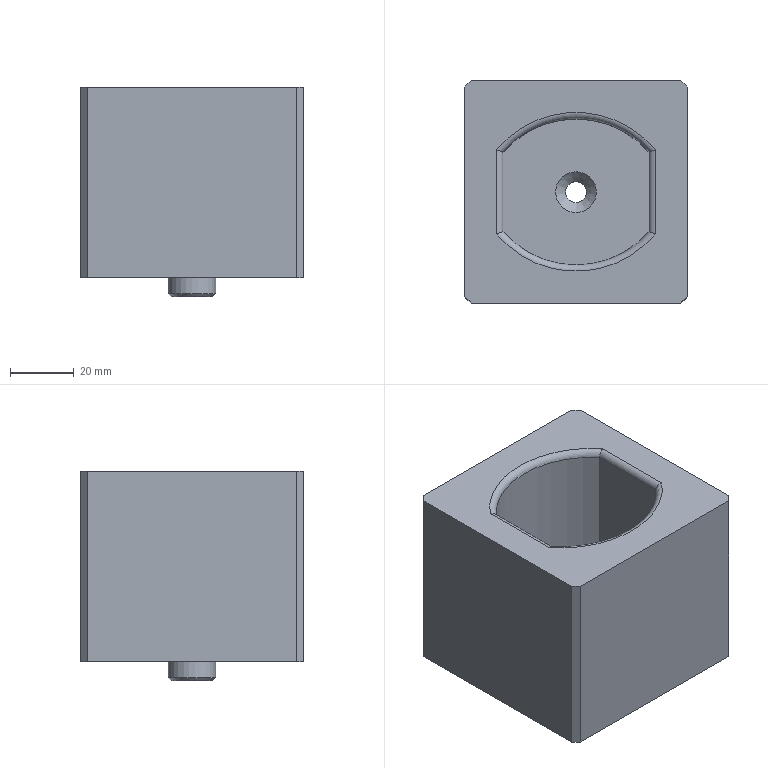NC program | NX | posted with a generic post | part box 70 x 70 x 66 mm
Lines 59 to 918 of 8582:
(ZLEVEL_PROFILE_COPY_1_COPY , TOOL : D16)
N116 T22 M6
N118 G54
N120 G17 G0 G90 X-8. Y-5.119 S7500 M3
N122 G43 Z30. H22
N124 Z1.4
N126 G94 G1 Y-5.61 Z1.374 F1000.
N128 X-8.004 Y-5.764 Z1.366
N130 X-7.18 Y-6.263 Z1.316
N132 X-4.893 Y-7.236 Z1.185
N134 X-2.48 Y-7.83 Z1.055
N136 X-0.002 Y-8.03 Z0.925
N138 X2.475 Y-7.83 Z0.795
N140 X4.889 Y-7.237 Z0.664
N142 X7.176 Y-6.265 Z0.534
N144 X8. Y-5.766 Z0.484
N146 Y5.764 Z-0.121
N148 X7.912 Y5.819 Z-0.126
N150 X7.084 Y6.312 Z-0.176
N152 X4.825 Y7.258 Z-0.305
N154 X2.444 Y7.835 Z-0.433
N156 X0.002 Y8.03 Z-0.562
N158 X-2.441 Y7.836 Z-0.69
N160 X-4.822 Y7.259 Z-0.818
N162 X-7.082 Y6.314 Z-0.947
N164 X-7.909 Y5.821 Z-0.997
N166 X-8. Y5.764 F2500.
N168 Y-5.61
N170 X-8.004 Y-5.764
N172 G3 X8. Y-5.766 R15.443
N174 G1 Y5.764
N176 X7.912 Y5.819
N178 G3 X-7.909 Y5.821 R15.443
N180 G1 X-7.995 Y5.764 Z-1.
N182 X-8. Y4.542 Z-1.028
N184 Y-4.76 Z-1.247
N186 X-7.983 Y-5.771 Z-1.27
N188 X-7.722 Y-5.927 Z-1.278
N190 X-7.137 Y-6.241 Z-1.293
N192 X-6.545 Y-6.543 Z-1.309
N194 X-5.937 Y-6.811 Z-1.325
N196 X-5.318 Y-7.051 Z-1.34
N198 X-4.688 Y-7.261 Z-1.356
N200 X-4.054 Y-7.459 Z-1.371
N202 X-3.408 Y-7.616 Z-1.387
N204 X-2.757 Y-7.746 Z-1.402
N206 X-2.1 Y-7.846 Z-1.418
N208 X-1.442 Y-7.933 Z-1.434
N210 X-0.779 Y-7.975 Z-1.449
N212 X-0.115 Y-7.993 Z-1.465
N214 X0.55 Y-7.981 Z-1.48
N216 X1.213 Y-7.952 Z-1.496
N218 X1.873 Y-7.877 Z-1.511
N220 X2.531 Y-7.784 Z-1.527
N222 X3.184 Y-7.661 Z-1.543
N224 X3.832 Y-7.516 Z-1.558
N226 X4.469 Y-7.33 Z-1.574
N228 X5.102 Y-7.128 Z-1.589
N230 X5.724 Y-6.895 Z-1.605
N232 X6.336 Y-6.638 Z-1.621
N234 X7.41 Y-6.101 Z-1.649
N236 X7.524 Y-6.041 Z-1.652
N238 X7.976 Y-5.776 Z-1.664
N240 X8. Y-4.987 Z-1.683
N242 Y5.644 Z-1.932
N244 Y5.761 Z-1.935
N246 X7.608 Y5.993 Z-1.946
N248 X6.939 Y6.343 Z-1.963
N250 X6.342 Y6.635 Z-1.979
N252 X5.732 Y6.896 Z-1.995
N254 G3 X-7.909 Y5.821 R15.443
N256 G1 X-7.995 Y5.764 Z-1.997
N258 X-8. Y4.542 Z-2.026
N260 Y-4.76 Z-2.244
N262 X-7.983 Y-5.771 Z-2.268
N264 X-7.722 Y-5.927 Z-2.275
N266 X-7.137 Y-6.241 Z-2.291
N268 X-6.545 Y-6.542 Z-2.306
N270 X-5.937 Y-6.811 Z-2.322
N272 X-5.318 Y-7.05 Z-2.337
N274 X-4.688 Y-7.261 Z-2.353
N276 X-4.053 Y-7.458 Z-2.369
N278 X-3.408 Y-7.616 Z-2.384
N280 X-2.757 Y-7.746 Z-2.4
N282 X-2.1 Y-7.845 Z-2.415
N284 X-1.441 Y-7.933 Z-2.431
N286 X-0.779 Y-7.975 Z-2.446
N288 X-0.115 Y-7.993 Z-2.462
N290 X0.55 Y-7.981 Z-2.478
N292 X1.213 Y-7.951 Z-2.493
N294 X1.873 Y-7.878 Z-2.509
N296 X2.531 Y-7.784 Z-2.524
N298 X3.183 Y-7.661 Z-2.54
N300 X3.832 Y-7.515 Z-2.556
N302 X4.469 Y-7.33 Z-2.571
N304 X5.102 Y-7.128 Z-2.587
N306 X5.724 Y-6.895 Z-2.602
N308 X6.336 Y-6.638 Z-2.618
N310 X7.41 Y-6.101 Z-2.646
N312 X7.524 Y-6.041 Z-2.649
N314 X7.975 Y-5.776 Z-2.662
N316 X8. Y-4.987 Z-2.68
N318 Y5.644 Z-2.929
N320 Y5.761 Z-2.932
N322 X7.608 Y5.993 Z-2.943
N324 X6.939 Y6.343 Z-2.961
N326 X6.342 Y6.635 Z-2.976
N328 X5.732 Y6.897 Z-2.992
N330 G3 X-7.909 Y5.821 R15.44
N332 G1 X-7.995 Y5.764 Z-2.994
N334 X-8. Y4.543 Z-3.023
N336 Y-4.76 Z-3.241
N338 X-7.984 Y-5.77 Z-3.265
N340 X-7.722 Y-5.926 Z-3.272
N342 X-7.137 Y-6.241 Z-3.288
N344 X-6.545 Y-6.542 Z-3.303
N346 X-5.937 Y-6.811 Z-3.319
N348 X-5.318 Y-7.05 Z-3.335
N350 X-4.688 Y-7.261 Z-3.35
N352 X-4.054 Y-7.458 Z-3.366
N354 X-3.408 Y-7.614 Z-3.381
N356 X-2.757 Y-7.746 Z-3.397
N358 X-2.1 Y-7.845 Z-3.413
N360 X-1.442 Y-7.933 Z-3.428
N362 X-0.779 Y-7.975 Z-3.444
N364 X-0.115 Y-7.993 Z-3.459
N366 X0.549 Y-7.981 Z-3.475
N368 X1.213 Y-7.952 Z-3.49
N370 X1.873 Y-7.877 Z-3.506
N372 X2.531 Y-7.784 Z-3.522
N374 X3.183 Y-7.661 Z-3.537
N376 X3.831 Y-7.516 Z-3.553
N378 X4.469 Y-7.33 Z-3.568
N380 X5.102 Y-7.128 Z-3.584
N382 X5.724 Y-6.895 Z-3.6
N384 X6.336 Y-6.638 Z-3.615
N386 X7.41 Y-6.101 Z-3.643
N388 X7.524 Y-6.041 Z-3.646
N390 X7.825 Y-5.865 Z-3.655
N392 X8. Y-5.761 Z-3.659
N394 Y-5.523 Z-3.665
N396 Y-4.987 Z-3.677
N398 Y5.645 Z-3.927
N400 Y5.761 Z-3.929
N402 X7.609 Y5.993 Z-3.94
N404 X6.939 Y6.342 Z-3.958
N406 X6.343 Y6.635 Z-3.974
N408 X5.732 Y6.897 Z-3.989
N410 G3 X-7.909 Y5.821 R15.44
N412 G1 X-7.997 Y5.763 Z-3.992
N414 X-8. Y4.543 Z-4.02
N416 Y-4.76 Z-4.238
N418 X-7.984 Y-5.77 Z-4.262
N420 X-7.722 Y-5.926 Z-4.27
N422 X-7.137 Y-6.241 Z-4.285
N424 X-6.545 Y-6.542 Z-4.301
N426 X-5.937 Y-6.811 Z-4.316
N428 X-5.318 Y-7.05 Z-4.332
N430 X-4.688 Y-7.261 Z-4.347
N432 X-4.054 Y-7.458 Z-4.363
N434 X-3.408 Y-7.614 Z-4.379
N436 X-2.757 Y-7.746 Z-4.394
N438 X-2.1 Y-7.845 Z-4.41
N440 X-1.442 Y-7.933 Z-4.425
N442 X-0.779 Y-7.975 Z-4.441
N444 X-0.115 Y-7.993 Z-4.457
N446 X0.55 Y-7.981 Z-4.472
N448 X1.213 Y-7.951 Z-4.488
N450 X1.873 Y-7.878 Z-4.503
N452 X2.531 Y-7.784 Z-4.519
N454 X3.183 Y-7.661 Z-4.534
N456 X3.831 Y-7.516 Z-4.55
N458 X4.469 Y-7.33 Z-4.566
N460 X5.102 Y-7.128 Z-4.581
N462 X5.724 Y-6.895 Z-4.597
N464 X6.336 Y-6.638 Z-4.612
N466 X7.41 Y-6.101 Z-4.641
N468 X7.524 Y-6.041 Z-4.644
N470 X7.825 Y-5.865 Z-4.652
N472 X8. Y-5.761 Z-4.657
N474 Y-5.523 Z-4.662
N476 Y-4.987 Z-4.675
N478 Y5.645 Z-4.924
N480 Y5.761 Z-4.927
N482 X7.609 Y5.993 Z-4.938
N484 X6.939 Y6.342 Z-4.955
N486 X6.342 Y6.635 Z-4.971
N488 X5.732 Y6.897 Z-4.986
N490 G3 X-7.909 Y5.821 R15.44
N492 G1 X-7.997 Y5.763 Z-4.989
N494 X-8. Y4.543 Z-5.018
N496 Y-4.76 Z-5.236
N498 X-7.984 Y-5.77 Z-5.26
N500 X-7.722 Y-5.926 Z-5.267
N502 X-7.137 Y-6.241 Z-5.282
N504 X-6.545 Y-6.542 Z-5.298
N506 X-5.937 Y-6.811 Z-5.314
N508 X-5.318 Y-7.05 Z-5.329
N510 X-4.688 Y-7.261 Z-5.345
N512 X-4.053 Y-7.458 Z-5.36
N514 X-3.408 Y-7.616 Z-5.376
N516 X-2.757 Y-7.746 Z-5.392
N518 X-2.1 Y-7.845 Z-5.407
N520 X-1.441 Y-7.933 Z-5.423
N522 X-0.779 Y-7.975 Z-5.438
N524 X-0.115 Y-7.993 Z-5.454
N526 X0.55 Y-7.981 Z-5.469
N528 X1.213 Y-7.951 Z-5.485
N530 X1.873 Y-7.877 Z-5.501
N532 X2.531 Y-7.784 Z-5.516
N534 X3.183 Y-7.661 Z-5.532
N536 X3.831 Y-7.515 Z-5.547
N538 X4.469 Y-7.33 Z-5.563
N540 X5.102 Y-7.128 Z-5.578
N542 X5.724 Y-6.895 Z-5.594
N544 X6.336 Y-6.638 Z-5.61
N546 X7.41 Y-6.101 Z-5.638
N548 X7.524 Y-6.041 Z-5.641
N550 X7.824 Y-5.865 Z-5.649
N552 X8. Y-5.761 Z-5.654
N554 Y-5.524 Z-5.66
N556 Y-4.987 Z-5.672
N558 Y5.645 Z-5.921
N560 Y5.761 Z-5.924
N562 X7.609 Y5.993 Z-5.935
N564 X6.939 Y6.342 Z-5.952
N566 X6.342 Y6.635 Z-5.968
N568 X5.732 Y6.897 Z-5.984
N570 G3 X-7.909 Y5.821 R15.44
N572 G1 X-7.997 Y5.763 Z-5.986
N574 X-8. Y4.543 Z-6.015
N576 Y-4.76 Z-6.233
N578 X-7.984 Y-5.77 Z-6.257
N580 X-7.721 Y-5.926 Z-6.264
N582 X-7.137 Y-6.241 Z-6.28
N584 X-6.545 Y-6.542 Z-6.295
N586 X-5.937 Y-6.81 Z-6.311
N588 X-5.318 Y-7.05 Z-6.326
N590 X-4.688 Y-7.261 Z-6.342
N592 X-4.053 Y-7.458 Z-6.358
N594 X-3.408 Y-7.616 Z-6.373
N596 X-2.757 Y-7.746 Z-6.389
N598 X-2.1 Y-7.845 Z-6.404
N600 X-1.441 Y-7.933 Z-6.42
N602 X-0.779 Y-7.975 Z-6.436
N604 X-0.115 Y-7.993 Z-6.451
N606 X0.55 Y-7.981 Z-6.467
N608 X1.213 Y-7.951 Z-6.482
N610 X1.873 Y-7.877 Z-6.498
N612 X2.531 Y-7.784 Z-6.513
N614 X3.184 Y-7.661 Z-6.529
N616 X3.832 Y-7.515 Z-6.545
N618 X4.469 Y-7.33 Z-6.56
N620 X5.102 Y-7.128 Z-6.576
N622 X5.724 Y-6.895 Z-6.591
N624 X6.336 Y-6.637 Z-6.607
N626 X7.41 Y-6.101 Z-6.635
N628 X7.524 Y-6.041 Z-6.638
N630 X7.824 Y-5.865 Z-6.646
N632 X8. Y-5.761 Z-6.651
N634 Y-5.524 Z-6.657
N636 Y-4.987 Z-6.669
N638 Y5.645 Z-6.919
N640 Y5.761 Z-6.921
N642 X7.609 Y5.993 Z-6.932
N644 X6.939 Y6.342 Z-6.95
N646 X6.342 Y6.635 Z-6.965
N648 X5.732 Y6.897 Z-6.981
N650 G3 X-7.909 Y5.821 R15.44
N652 G1 X-7.997 Y5.763 Z-6.983
N654 X-8. Y4.543 Z-7.012
N656 Y-4.76 Z-7.23
N658 X-7.984 Y-5.77 Z-7.254
N660 X-7.721 Y-5.926 Z-7.261
N662 X-7.137 Y-6.241 Z-7.277
N664 X-6.545 Y-6.542 Z-7.293
N666 X-5.937 Y-6.81 Z-7.308
N668 X-5.317 Y-7.05 Z-7.324
N670 X-4.688 Y-7.261 Z-7.339
N672 X-4.053 Y-7.458 Z-7.355
N674 X-3.408 Y-7.616 Z-7.37
N676 X-2.757 Y-7.746 Z-7.386
N678 X-2.1 Y-7.845 Z-7.402
N680 X-1.441 Y-7.933 Z-7.417
N682 X-0.779 Y-7.975 Z-7.433
N684 X-0.114 Y-7.993 Z-7.448
N686 X0.55 Y-7.981 Z-7.464
N688 X1.213 Y-7.951 Z-7.48
N690 X1.873 Y-7.877 Z-7.495
N692 X2.531 Y-7.784 Z-7.511
N694 X3.184 Y-7.661 Z-7.526
N696 X3.832 Y-7.515 Z-7.542
N698 X4.469 Y-7.33 Z-7.557
N700 X5.102 Y-7.128 Z-7.573
N702 X5.724 Y-6.895 Z-7.589
N704 X6.336 Y-6.637 Z-7.604
N706 X7.41 Y-6.101 Z-7.632
N708 X7.524 Y-6.041 Z-7.635
N710 X7.824 Y-5.865 Z-7.644
N712 X8. Y-5.761 Z-7.649
N714 Y-5.524 Z-7.654
N716 Y-4.987 Z-7.667
N718 Y5.645 Z-7.916
N720 Y5.761 Z-7.919
N722 X7.609 Y5.993 Z-7.929
N724 X6.939 Y6.342 Z-7.947
N726 X6.342 Y6.635 Z-7.963
N728 X5.732 Y6.897 Z-7.978
N730 G3 X-7.909 Y5.821 R15.44
N732 G1 X-7.997 Y5.763 Z-7.981
N734 X-8. Y4.543 Z-8.009
N736 Y-4.76 Z-8.228
N738 X-7.984 Y-5.77 Z-8.251
N740 X-7.721 Y-5.926 Z-8.259
N742 X-7.137 Y-6.241 Z-8.274
N744 X-6.545 Y-6.542 Z-8.29
N746 X-5.937 Y-6.81 Z-8.305
N748 X-5.317 Y-7.05 Z-8.321
N750 X-4.688 Y-7.261 Z-8.337
N752 X-4.053 Y-7.458 Z-8.352
N754 X-3.408 Y-7.616 Z-8.368
N756 X-2.757 Y-7.746 Z-8.383
N758 X-2.1 Y-7.845 Z-8.399
N760 X-1.441 Y-7.933 Z-8.414
N762 X-0.778 Y-7.975 Z-8.43
N764 X-0.114 Y-7.993 Z-8.446
N766 X0.55 Y-7.981 Z-8.461
N768 X1.213 Y-7.951 Z-8.477
N770 X1.873 Y-7.877 Z-8.492
N772 X2.531 Y-7.784 Z-8.508
N774 X3.184 Y-7.661 Z-8.524
N776 X3.832 Y-7.515 Z-8.539
N778 X4.469 Y-7.33 Z-8.555
N780 X5.102 Y-7.128 Z-8.57
N782 X5.724 Y-6.894 Z-8.586
N784 X6.336 Y-6.637 Z-8.601
N786 X7.41 Y-6.101 Z-8.63
N788 X7.524 Y-6.041 Z-8.633
N790 X7.824 Y-5.865 Z-8.641
N792 X8. Y-5.76 Z-8.646
N794 Y-5.524 Z-8.651
N796 Y-4.987 Z-8.664
N798 Y5.645 Z-8.913
N800 Y5.761 Z-8.916
N802 X7.609 Y5.993 Z-8.927
N804 X6.939 Y6.342 Z-8.944
N806 X6.342 Y6.635 Z-8.96
N808 X5.732 Y6.897 Z-8.975
N810 G3 X-7.909 Y5.821 R15.44
N812 G1 X-7.996 Y5.763 Z-8.978
N814 X-8. Y4.543 Z-9.007
N816 Y-4.76 Z-9.225
N818 X-7.984 Y-5.77 Z-9.249
N820 X-7.721 Y-5.926 Z-9.256
N822 X-7.137 Y-6.241 Z-9.272
N824 X-6.545 Y-6.542 Z-9.287
N826 X-5.937 Y-6.81 Z-9.303
N828 X-5.317 Y-7.05 Z-9.318
N830 X-4.687 Y-7.261 Z-9.334
N832 X-4.053 Y-7.458 Z-9.349
N834 X-3.408 Y-7.616 Z-9.365
N836 X-2.757 Y-7.746 Z-9.381
N838 X-2.1 Y-7.845 Z-9.396
N840 X-1.441 Y-7.933 Z-9.412
N842 X-0.778 Y-7.974 Z-9.427
N844 X-0.114 Y-7.993 Z-9.443
N846 X0.55 Y-7.981 Z-9.459
N848 X1.213 Y-7.951 Z-9.474
N850 X1.873 Y-7.877 Z-9.49
N852 X2.531 Y-7.783 Z-9.505
N854 X3.184 Y-7.661 Z-9.521
N856 X3.832 Y-7.515 Z-9.536
N858 X4.469 Y-7.33 Z-9.552
N860 X5.102 Y-7.128 Z-9.568
N862 X5.724 Y-6.894 Z-9.583
N864 X6.336 Y-6.637 Z-9.599
N866 X7.41 Y-6.101 Z-9.627
N868 X7.524 Y-6.041 Z-9.63
N870 X7.824 Y-5.865 Z-9.638
N872 X8. Y-5.76 Z-9.643
N874 Y-5.524 Z-9.649
N876 Y-4.987 Z-9.661
N878 Y5.645 Z-9.91
N880 Y5.761 Z-9.913
N882 X7.608 Y5.993 Z-9.924
N884 X6.939 Y6.342 Z-9.942
N886 X6.342 Y6.635 Z-9.957
N888 X5.732 Y6.897 Z-9.973
N890 G3 X-7.909 Y5.821 R15.44
N892 G1 X-7.996 Y5.763 Z-9.975
N894 X-8. Y4.543 Z-10.004
N896 Y-4.76 Z-10.222
N898 X-7.984 Y-5.77 Z-10.246
N900 X-7.721 Y-5.926 Z-10.253
N902 X-7.137 Y-6.241 Z-10.269
N904 X-6.544 Y-6.542 Z-10.284
N906 X-5.937 Y-6.81 Z-10.3
N908 X-5.317 Y-7.05 Z-10.316
N910 X-4.687 Y-7.261 Z-10.331
N912 X-4.053 Y-7.459 Z-10.347
N914 X-3.408 Y-7.616 Z-10.362
N916 X-2.756 Y-7.746 Z-10.378
N918 X-2.1 Y-7.845 Z-10.393
N920 X-1.441 Y-7.933 Z-10.409
N922 X-0.778 Y-7.974 Z-10.425
N924 X-0.114 Y-7.993 Z-10.44
N926 X0.55 Y-7.981 Z-10.456
N928 X1.213 Y-7.951 Z-10.471
N930 X1.873 Y-7.877 Z-10.487
N932 X2.531 Y-7.783 Z-10.503
N934 X3.184 Y-7.661 Z-10.518
N936 X3.832 Y-7.515 Z-10.534
N938 X4.469 Y-7.33 Z-10.549
N940 X5.102 Y-7.128 Z-10.565
N942 X5.724 Y-6.894 Z-10.58
N944 X6.336 Y-6.637 Z-10.596
N946 X7.41 Y-6.101 Z-10.624
N948 X7.524 Y-6.041 Z-10.627
N950 X7.824 Y-5.865 Z-10.635
N952 X8. Y-5.76 Z-10.64
N954 Y-5.524 Z-10.646
N956 Y-4.987 Z-10.658
N958 Y5.645 Z-10.908
N960 Y5.761 Z-10.91
N962 X7.608 Y5.993 Z-10.921
N964 X6.939 Y6.342 Z-10.939
N966 X6.342 Y6.635 Z-10.954
N968 X5.732 Y6.897 Z-10.97
N970 G3 X-7.909 Y5.821 R15.44
N972 G1 X-7.996 Y5.762 Z-10.973
N974 X-8. Y4.543 Z-11.001
N976 Y-4.76 Z-11.219
N978 X-7.984 Y-5.77 Z-11.243
N980 X-7.721 Y-5.926 Z-11.25
N982 X-7.137 Y-6.241 Z-11.266
N984 X-6.544 Y-6.542 Z-11.282
N986 X-5.937 Y-6.81 Z-11.297
N988 X-5.317 Y-7.05 Z-11.313
N990 X-4.687 Y-7.261 Z-11.328
N992 X-4.053 Y-7.459 Z-11.344
N994 X-3.408 Y-7.616 Z-11.36
N996 X-2.756 Y-7.746 Z-11.375
N998 X-2.1 Y-7.845 Z-11.391
N1000 X-1.441 Y-7.933 Z-11.406
N1002 X-0.778 Y-7.974 Z-11.422
N1004 X-0.114 Y-7.993 Z-11.437
N1006 X0.55 Y-7.981 Z-11.453
N1008 X1.213 Y-7.951 Z-11.469
N1010 X1.873 Y-7.877 Z-11.484
N1012 X2.531 Y-7.783 Z-11.5
N1014 X3.184 Y-7.661 Z-11.515
N1016 X3.832 Y-7.515 Z-11.531
N1018 X4.469 Y-7.33 Z-11.547
N1020 X5.102 Y-7.128 Z-11.562
N1022 X5.724 Y-6.894 Z-11.578
N1024 X6.336 Y-6.637 Z-11.593
N1026 X7.41 Y-6.101 Z-11.621
N1028 X7.524 Y-6.041 Z-11.624
N1030 X7.824 Y-5.865 Z-11.633
N1032 X8. Y-5.76 Z-11.638
N1034 Y-5.524 Z-11.643
N1036 Y-4.987 Z-11.656
N1038 Y5.645 Z-11.905
N1040 Y5.76 Z-11.908
N1042 X7.608 Y5.993 Z-11.918
N1044 X6.939 Y6.342 Z-11.936
N1046 X6.342 Y6.635 Z-11.952
N1048 X5.732 Y6.897 Z-11.967
N1050 G3 X-7.909 Y5.821 R15.44
N1052 G1 X-7.996 Y5.762 Z-11.97
N1054 X-8. Y4.543 Z-11.998
N1056 Y-4.76 Z-12.217
N1058 X-7.984 Y-5.77 Z-12.24
N1060 X-7.721 Y-5.926 Z-12.248
N1062 X-7.137 Y-6.241 Z-12.263
N1064 X-6.544 Y-6.542 Z-12.279
N1066 X-5.937 Y-6.81 Z-12.295
N1068 X-5.317 Y-7.05 Z-12.31
N1070 X-4.687 Y-7.261 Z-12.326
N1072 X-4.053 Y-7.459 Z-12.341
N1074 X-3.408 Y-7.616 Z-12.357
N1076 X-2.756 Y-7.746 Z-12.372
N1078 X-2.1 Y-7.845 Z-12.388
N1080 X-1.441 Y-7.933 Z-12.404
N1082 X-0.778 Y-7.974 Z-12.419
N1084 X-0.114 Y-7.992 Z-12.435
N1086 X0.55 Y-7.981 Z-12.45
N1088 X1.213 Y-7.951 Z-12.466
N1090 X1.873 Y-7.877 Z-12.481
N1092 X2.531 Y-7.783 Z-12.497
N1094 X3.184 Y-7.661 Z-12.513
N1096 X3.832 Y-7.515 Z-12.528
N1098 X4.469 Y-7.33 Z-12.544
N1100 X5.102 Y-7.128 Z-12.559
N1102 X5.724 Y-6.894 Z-12.575
N1104 X6.336 Y-6.637 Z-12.591
N1106 X7.41 Y-6.101 Z-12.619
N1108 X7.524 Y-6.041 Z-12.622
N1110 X7.824 Y-5.865 Z-12.63
N1112 X8. Y-5.76 Z-12.635
N1114 Y-5.525 Z-12.64
N1116 Y-4.987 Z-12.653
N1118 Y5.645 Z-12.902
N1120 Y5.76 Z-12.905
N1122 X7.608 Y5.993 Z-12.916
N1124 X6.939 Y6.342 Z-12.933
N1126 X6.342 Y6.635 Z-12.949
N1128 X5.732 Y6.897 Z-12.965
N1130 G3 X-7.909 Y5.821 R15.44
N1132 G1 X-7.996 Y5.762 Z-12.967
N1134 X-8. Y4.543 Z-12.996
N1136 Y-4.76 Z-13.214
N1138 X-7.984 Y-5.77 Z-13.238
N1140 X-7.721 Y-5.926 Z-13.245
N1142 X-7.136 Y-6.241 Z-13.261
N1144 X-6.544 Y-6.542 Z-13.276
N1146 X-5.937 Y-6.811 Z-13.292
N1148 X-5.317 Y-7.05 Z-13.307
N1150 X-4.687 Y-7.261 Z-13.323
N1152 X-4.053 Y-7.459 Z-13.339
N1154 X-3.408 Y-7.616 Z-13.354
N1156 X-2.756 Y-7.746 Z-13.37
N1158 X-2.099 Y-7.845 Z-13.385
N1160 X-1.441 Y-7.933 Z-13.401
N1162 X-0.778 Y-7.974 Z-13.416
N1164 X-0.114 Y-7.992 Z-13.432
N1166 X0.55 Y-7.981 Z-13.448
N1168 X1.213 Y-7.951 Z-13.463
N1170 X1.873 Y-7.877 Z-13.479
N1172 X2.531 Y-7.783 Z-13.494
N1174 X3.184 Y-7.661 Z-13.51
N1176 X3.832 Y-7.515 Z-13.526
N1178 X4.469 Y-7.329 Z-13.541
N1180 X5.102 Y-7.128 Z-13.557
N1182 X5.724 Y-6.894 Z-13.572
N1184 X6.336 Y-6.637 Z-13.588
N1186 X7.41 Y-6.101 Z-13.616
N1188 X7.524 Y-6.041 Z-13.619
N1190 X7.823 Y-5.865 Z-13.627
N1192 X8. Y-5.761 Z-13.632
N1194 Y-5.525 Z-13.638
N1196 Y-4.987 Z-13.65
N1198 Y5.645 Z-13.899
N1200 Y5.76 Z-13.902
N1202 X7.608 Y5.992 Z-13.913
N1204 X6.939 Y6.342 Z-13.931
N1206 X6.342 Y6.635 Z-13.946
N1208 X5.732 Y6.897 Z-13.962
N1210 G3 X-7.909 Y5.821 R15.44
N1212 G1 X-7.996 Y5.762 Z-13.964
N1214 X-8. Y4.542 Z-13.993
N1216 Y-4.76 Z-14.211
N1218 X-7.984 Y-5.77 Z-14.235
N1220 X-7.721 Y-5.926 Z-14.242
N1222 X-7.136 Y-6.241 Z-14.258
N1224 X-6.544 Y-6.542 Z-14.273
N1226 X-5.937 Y-6.811 Z-14.289
N1228 X-5.317 Y-7.05 Z-14.305
N1230 X-4.687 Y-7.261 Z-14.32
N1232 X-4.053 Y-7.459 Z-14.336
N1234 X-3.408 Y-7.616 Z-14.351
N1236 X-2.756 Y-7.746 Z-14.367
N1238 X-2.099 Y-7.845 Z-14.383
N1240 X-1.441 Y-7.933 Z-14.398
N1242 X-0.778 Y-7.974 Z-14.414
N1244 X-0.114 Y-7.992 Z-14.429
N1246 X0.55 Y-7.981 Z-14.445
N1248 X1.213 Y-7.951 Z-14.46
N1250 X1.873 Y-7.877 Z-14.476
N1252 X2.531 Y-7.783 Z-14.492
N1254 X3.184 Y-7.661 Z-14.507
N1256 X3.832 Y-7.515 Z-14.523
N1258 X4.469 Y-7.329 Z-14.538
N1260 X5.102 Y-7.128 Z-14.554
N1262 X5.724 Y-6.894 Z-14.57
N1264 X6.336 Y-6.637 Z-14.585
N1266 X7.41 Y-6.101 Z-14.613
N1268 X7.524 Y-6.041 Z-14.616
N1270 X7.823 Y-5.865 Z-14.625
N1272 X8. Y-5.76 Z-14.629
N1274 Y-5.525 Z-14.635
N1276 Y-4.987 Z-14.647
N1278 Y5.645 Z-14.897
N1280 Y5.76 Z-14.899
N1282 X7.608 Y5.992 Z-14.91
N1284 X6.939 Y6.342 Z-14.928
N1286 X6.342 Y6.634 Z-14.944
N1288 X5.732 Y6.897 Z-14.959
N1290 G3 X-7.909 Y5.821 R15.44
N1292 G1 X-7.996 Y5.762 Z-14.962
N1294 X-8. Y4.542 Z-14.99
N1296 Y-4.76 Z-15.208
N1298 X-7.984 Y-5.77 Z-15.232
N1300 X-7.721 Y-5.926 Z-15.24
N1302 X-7.136 Y-6.241 Z-15.255
N1304 X-6.544 Y-6.542 Z-15.271
N1306 X-5.937 Y-6.811 Z-15.286
N1308 X-5.317 Y-7.05 Z-15.302
N1310 X-4.687 Y-7.261 Z-15.317
N1312 X-4.053 Y-7.459 Z-15.333
N1314 X-3.408 Y-7.616 Z-15.349
N1316 X-2.756 Y-7.746 Z-15.364
N1318 X-2.099 Y-7.845 Z-15.38
N1320 X-1.441 Y-7.933 Z-15.395
N1322 X-0.778 Y-7.974 Z-15.411
N1324 X-0.114 Y-7.992 Z-15.427
N1326 X0.55 Y-7.98 Z-15.442
N1328 X1.213 Y-7.951 Z-15.458
N1330 X1.873 Y-7.876 Z-15.473
N1332 X2.531 Y-7.783 Z-15.489
N1334 X3.184 Y-7.66 Z-15.504
N1336 X3.832 Y-7.515 Z-15.52
N1338 X4.469 Y-7.329 Z-15.536
N1340 X5.102 Y-7.128 Z-15.551
N1342 X5.724 Y-6.894 Z-15.567
N1344 X6.336 Y-6.637 Z-15.582
N1346 X7.41 Y-6.101 Z-15.611
N1348 X7.524 Y-6.041 Z-15.614
N1350 X7.823 Y-5.865 Z-15.622
N1352 X8. Y-5.76 Z-15.627
N1354 Y-5.525 Z-15.632
N1356 Y-4.987 Z-15.645
N1358 Y5.645 Z-15.894
N1360 Y5.76 Z-15.897
N1362 X7.608 Y5.992 Z-15.908
N1364 X6.939 Y6.342 Z-15.925
N1366 X6.342 Y6.634 Z-15.941
N1368 X5.732 Y6.897 Z-15.956
N1370 G3 X-7.909 Y5.821 R15.44
N1372 G1 X-7.996 Y5.762 Z-15.959
N1374 X-8. Y4.542 Z-15.988
N1376 Y-4.76 Z-16.206
N1378 X-7.984 Y-5.77 Z-16.229
N1380 X-7.721 Y-5.926 Z-16.237
N1382 X-7.136 Y-6.241 Z-16.252
N1384 X-6.544 Y-6.542 Z-16.268
N1386 X-5.937 Y-6.811 Z-16.284
N1388 X-5.317 Y-7.05 Z-16.299
N1390 X-4.687 Y-7.261 Z-16.315
N1392 X-4.053 Y-7.459 Z-16.33
N1394 X-3.408 Y-7.616 Z-16.346
N1396 X-2.756 Y-7.746 Z-16.362
N1398 X-2.099 Y-7.845 Z-16.377
N1400 X-1.441 Y-7.933 Z-16.393
N1402 X-0.778 Y-7.974 Z-16.408
N1404 X-0.114 Y-7.992 Z-16.424
N1406 X0.55 Y-7.98 Z-16.439
N1408 X1.213 Y-7.951 Z-16.455
N1410 X1.873 Y-7.876 Z-16.471
N1412 X2.531 Y-7.783 Z-16.486
N1414 X3.184 Y-7.66 Z-16.502
N1416 X3.832 Y-7.515 Z-16.517
N1418 X4.469 Y-7.329 Z-16.533
N1420 X5.102 Y-7.128 Z-16.548
N1422 X5.724 Y-6.894 Z-16.564
N1424 X6.337 Y-6.637 Z-16.58
N1426 X7.409 Y-6.1 Z-16.608
N1428 X7.524 Y-6.041 Z-16.611
N1430 X7.823 Y-5.865 Z-16.619
N1432 X8. Y-5.76 Z-16.624
N1434 Y-5.525 Z-16.63
N1436 Y-4.987 Z-16.642
N1438 Y5.645 Z-16.891
N1440 Y5.76 Z-16.894
N1442 X7.608 Y5.992 Z-16.905
N1444 X6.939 Y6.342 Z-16.922
N1446 X6.342 Y6.634 Z-16.938
N1448 X5.732 Y6.897 Z-16.954
N1450 G3 X-7.909 Y5.821 R15.44
N1452 G1 X-7.996 Y5.762 Z-16.956
N1454 X-8. Y4.542 Z-16.985
N1456 Y-4.76 Z-17.203
N1458 X-7.984 Y-5.77 Z-17.227
N1460 X-7.721 Y-5.926 Z-17.234
N1462 X-7.136 Y-6.241 Z-17.25
N1464 X-6.544 Y-6.542 Z-17.265
N1466 X-5.937 Y-6.81 Z-17.281
N1468 X-5.317 Y-7.05 Z-17.296
N1470 X-4.687 Y-7.261 Z-17.312
N1472 X-4.053 Y-7.459 Z-17.328
N1474 X-3.408 Y-7.616 Z-17.343
N1476 X-2.756 Y-7.746 Z-17.359
N1478 X-2.099 Y-7.844 Z-17.374
N1480 X-1.441 Y-7.933 Z-17.39
N1482 X-0.778 Y-7.974 Z-17.406
N1484 X-0.114 Y-7.992 Z-17.421
N1486 X0.55 Y-7.98 Z-17.437
N1488 X1.213 Y-7.951 Z-17.452
N1490 X1.873 Y-7.876 Z-17.468
N1492 X2.531 Y-7.783 Z-17.483
N1494 X3.184 Y-7.66 Z-17.499
N1496 X3.832 Y-7.515 Z-17.515
N1498 X4.469 Y-7.329 Z-17.53
N1500 X5.102 Y-7.128 Z-17.546
N1502 X5.724 Y-6.894 Z-17.561
N1504 X6.337 Y-6.637 Z-17.577
N1506 X7.409 Y-6.1 Z-17.605
N1508 X7.524 Y-6.041 Z-17.608
N1510 X7.823 Y-5.865 Z-17.616
N1512 X8. Y-5.76 Z-17.621
N1514 Y-5.525 Z-17.627
N1516 Y-4.987 Z-17.639
N1518 Y5.645 Z-17.889
N1520 Y5.76 Z-17.891
N1522 X7.608 Y5.992 Z-17.902
N1524 X6.938 Y6.342 Z-17.92
N1526 X6.342 Y6.634 Z-17.935
N1528 X5.732 Y6.897 Z-17.951
N1530 G3 X-7.909 Y5.821 R15.44
N1532 G1 X-7.996 Y5.762 Z-17.953
N1534 X-8. Y4.542 Z-17.982
N1536 Y-4.76 Z-18.2
N1538 X-7.984 Y-5.77 Z-18.224
N1540 X-7.721 Y-5.926 Z-18.231
N1542 X-7.136 Y-6.241 Z-18.247
N1544 X-6.544 Y-6.542 Z-18.263
N1546 X-5.936 Y-6.81 Z-18.278
N1548 X-5.317 Y-7.05 Z-18.294
N1550 X-4.687 Y-7.261 Z-18.309
N1552 X-4.053 Y-7.459 Z-18.325
N1554 X-3.407 Y-7.615 Z-18.34
N1556 X-2.756 Y-7.746 Z-18.356
N1558 X-2.099 Y-7.844 Z-18.372
N1560 X-1.441 Y-7.933 Z-18.387
N1562 X-0.778 Y-7.974 Z-18.403
N1564 X-0.114 Y-7.992 Z-18.418
N1566 X0.55 Y-7.98 Z-18.434
N1568 X1.213 Y-7.951 Z-18.45
N1570 X1.873 Y-7.877 Z-18.465
N1572 X2.531 Y-7.783 Z-18.481
N1574 X3.184 Y-7.66 Z-18.496
N1576 X3.832 Y-7.515 Z-18.512
N1578 X4.47 Y-7.33 Z-18.527
N1580 X5.102 Y-7.128 Z-18.543
N1582 X5.724 Y-6.894 Z-18.559
N1584 X6.337 Y-6.637 Z-18.574
N1586 X7.409 Y-6.1 Z-18.602
N1588 X7.524 Y-6.041 Z-18.605
N1590 X7.822 Y-5.865 Z-18.614
N1592 X8. Y-5.76 Z-18.619
N1594 Y-5.525 Z-18.624
N1596 Y-4.987 Z-18.637
N1598 Y5.645 Z-18.886
N1600 Y5.76 Z-18.888
N1602 X7.608 Y5.992 Z-18.899
N1604 X6.938 Y6.342 Z-18.917
N1606 X6.342 Y6.634 Z-18.933
N1608 X5.732 Y6.897 Z-18.948
N1610 G3 X-7.909 Y5.821 R15.44
N1612 G1 X-7.996 Y5.762 Z-18.951
N1614 X-8. Y4.542 Z-18.979
N1616 Y-4.76 Z-19.198
N1618 X-7.984 Y-5.769 Z-19.221
N1620 X-7.721 Y-5.926 Z-19.229
N1622 X-7.136 Y-6.241 Z-19.244
N1624 X-6.544 Y-6.542 Z-19.26
N1626 X-5.936 Y-6.81 Z-19.275
N1628 X-5.317 Y-7.05 Z-19.291
N1630 X-4.687 Y-7.261 Z-19.307
N1632 X-4.053 Y-7.459 Z-19.322
N1634 X-3.407 Y-7.615 Z-19.338
N1636 X-2.756 Y-7.746 Z-19.353
N1638 X-2.099 Y-7.844 Z-19.369
N1640 X-1.441 Y-7.933 Z-19.384
N1642 X-0.778 Y-7.974 Z-19.4
N1644 X-0.114 Y-7.992 Z-19.416
N1646 X0.55 Y-7.98 Z-19.431
N1648 X1.214 Y-7.951 Z-19.447
N1650 X1.873 Y-7.877 Z-19.462
N1652 X2.531 Y-7.783 Z-19.478
N1654 X3.184 Y-7.66 Z-19.494
N1656 X3.832 Y-7.515 Z-19.509
N1658 X4.47 Y-7.33 Z-19.525
N1660 X5.102 Y-7.128 Z-19.54
N1662 X5.724 Y-6.894 Z-19.556
N1664 X6.337 Y-6.637 Z-19.571
N1666 X7.409 Y-6.1 Z-19.6
N1668 X7.524 Y-6.041 Z-19.603
N1670 X7.822 Y-5.866 Z-19.611
N1672 X8. Y-5.76 Z-19.616
N1674 Y-5.526 Z-19.621
N1676 Y-4.987 Z-19.634
N1678 Y5.645 Z-19.883
N1680 Y5.76 Z-19.886
N1682 X7.608 Y5.992 Z-19.897
N1684 X6.938 Y6.342 Z-19.914
N1686 X6.342 Y6.635 Z-19.93
N1688 X5.732 Y6.897 Z-19.945
N1690 G3 X-7.909 Y5.821 R15.44
N1692 G1 X-7.996 Y5.762 Z-19.948
N1694 X-8. Y4.542 Z-19.977
N1696 Y-4.76 Z-20.195
N1698 X-7.984 Y-5.77 Z-20.219
N1700 X-7.72 Y-5.926 Z-20.226
N1702 X-7.136 Y-6.241 Z-20.242
N1704 X-6.544 Y-6.542 Z-20.257
N1706 X-5.936 Y-6.81 Z-20.273
N1708 X-5.317 Y-7.05 Z-20.288
N1710 X-4.687 Y-7.26 Z-20.304
N1712 X-4.053 Y-7.459 Z-20.319
N1714 X-3.407 Y-7.615 Z-20.335
N1716 X-2.756 Y-7.746 Z-20.351
N1718 X-2.099 Y-7.844 Z-20.366
N1720 X-1.441 Y-7.933 Z-20.382
N1722 X-0.778 Y-7.974 Z-20.397
N1724 X-0.114 Y-7.992 Z-20.413
N1726 X0.55 Y-7.98 Z-20.429
N1728 X1.214 Y-7.951 Z-20.444
N1730 X1.874 Y-7.877 Z-20.46
N1732 X2.531 Y-7.783 Z-20.475
N1734 X3.184 Y-7.661 Z-20.491
N1736 X3.832 Y-7.515 Z-20.506
N1738 X4.47 Y-7.33 Z-20.522
N1740 X5.102 Y-7.128 Z-20.538
N1742 X5.724 Y-6.893 Z-20.553
N1744 X6.337 Y-6.637 Z-20.569
N1746 X7.409 Y-6.1 Z-20.597
N1748 X7.524 Y-6.041 Z-20.6
N1750 X7.822 Y-5.866 Z-20.608
N1752 X8.001 Y-5.76 Z-20.613
N1754 X8. Y-5.526 Z-20.619
N1756 Y-4.987 Z-20.631
N1758 Y5.645 Z-20.88
N1760 Y5.76 Z-20.883
N1762 X7.609 Y5.992 Z-20.894
N1764 X6.938 Y6.342 Z-20.912
N1766 X6.342 Y6.635 Z-20.927
N1768 X5.732 Y6.897 Z-20.943
N1770 G3 X-7.909 Y5.821 R15.44
N1772 G1 X-7.996 Y5.762 Z-20.945
N1774 X-8. Y4.542 Z-20.974
N1776 Y-4.76 Z-21.192
N1778 X-7.984 Y-5.77 Z-21.216
N1780 X-7.72 Y-5.926 Z-21.223
N1782 X-7.136 Y-6.241 Z-21.239
N1784 X-6.544 Y-6.542 Z-21.254
N1786 X-5.936 Y-6.81 Z-21.27
N1788 X-5.317 Y-7.05 Z-21.286
N1790 X-4.687 Y-7.26 Z-21.301
N1792 X-4.053 Y-7.459 Z-21.317
N1794 X-3.407 Y-7.615 Z-21.332
N1796 X-2.756 Y-7.746 Z-21.348
N1798 X-2.099 Y-7.844 Z-21.363
N1800 X-1.441 Y-7.933 Z-21.379
N1802 X-0.778 Y-7.974 Z-21.395
N1804 X-0.114 Y-7.992 Z-21.41
N1806 X0.55 Y-7.98 Z-21.426
N1808 X1.214 Y-7.951 Z-21.441
N1810 X1.874 Y-7.877 Z-21.457
N1812 X2.531 Y-7.783 Z-21.473
N1814 X3.184 Y-7.66 Z-21.488
N1816 X3.832 Y-7.515 Z-21.504
N1818 X4.47 Y-7.329 Z-21.519
N1820 X5.102 Y-7.128 Z-21.535
N1822 X5.724 Y-6.893 Z-21.55
N1824 X6.337 Y-6.637 Z-21.566
N1826 X7.409 Y-6.1 Z-21.594
N1828 X7.524 Y-6.041 Z-21.597